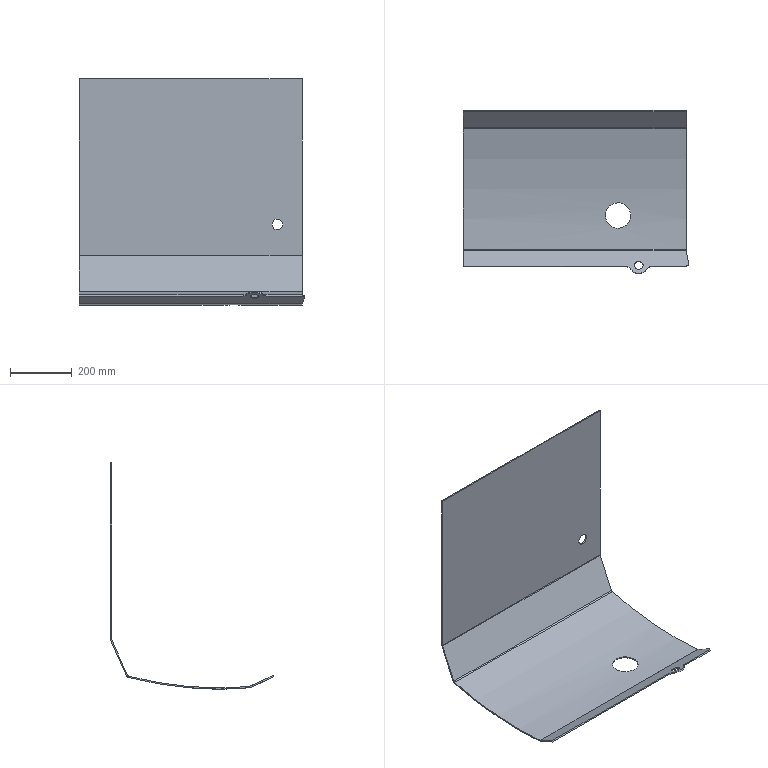Part | SolidWorks | features ICE 4, Fillet 1, FlatPattern 1, Fold 1, SMBaseFlange 1, SheetMetal 1, UnFold 1 | 1 solid | 41 faces | box 728.102 x 528.57 x 731.248 mm | volume 3316109 mm3 | plane 23 | cylinder 16 | spline 2 | commonest cylinder face diameters 20 x4 12 x3 29 x2 34 x2 40 x2 58 x1